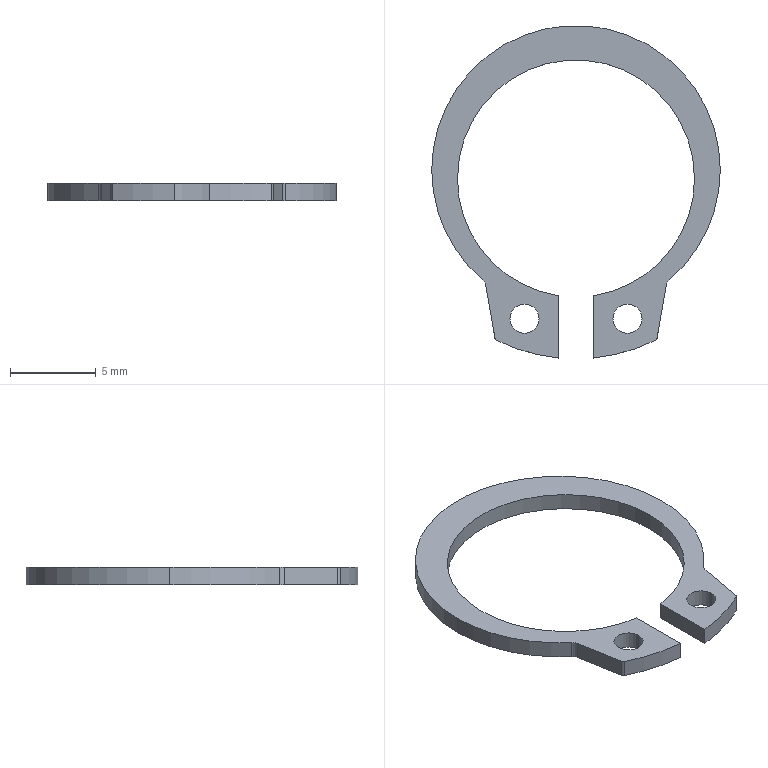Part | SolidWorks | features Fillet 2, Extrusion 1 | 1 solid | 22 faces | box 16.8 x 19.352 x 1 mm | volume 87.473 mm3 | cylinder 16 | plane 6 | commonest cylinder face diameters 1.7 x4 13.8 x3 16.8 x3 0.4 x2 1 x2 21 x2
STEP:
#1=CARTESIAN_POINT('',(2.15,-8.666,-1.));
#2=VERTEX_POINT('',#1);
#3=CARTESIAN_POINT('',(3.85,-8.666,-1.));
#4=VERTEX_POINT('',#3);
#5=CARTESIAN_POINT('',(3.,-8.666,-1.));
#6=DIRECTION('',(0.,0.,1.));
#7=DIRECTION('',(-1.,0.,0.));
#8=AXIS2_PLACEMENT_3D('',#5,#6,#7);
#9=CIRCLE('',#8,0.85);
#10=EDGE_CURVE('',#2,#4,#9,.T.);
#11=ORIENTED_EDGE('',*,*,#10,.F.);
#12=CARTESIAN_POINT('',(2.15,-8.666,0.));
#13=VERTEX_POINT('',#12);
#14=CARTESIAN_POINT('',(2.15,-8.666,-1.));
#15=DIRECTION('',(0.,0.,1.));
#16=VECTOR('',#15,1000.);
#17=LINE('',#14,#16);
#18=EDGE_CURVE('',#2,#13,#17,.T.);
#19=ORIENTED_EDGE('',*,*,#18,.T.);
#20=CARTESIAN_POINT('',(3.85,-8.666,0.));
#21=VERTEX_POINT('',#20);
#22=CARTESIAN_POINT('',(3.,-8.666,0.));
#23=DIRECTION('',(0.,0.,1.));
#24=DIRECTION('',(-1.,0.,0.));
#25=AXIS2_PLACEMENT_3D('',#22,#23,#24);
#26=CIRCLE('',#25,0.85);
#27=EDGE_CURVE('',#13,#21,#26,.T.);
#28=ORIENTED_EDGE('',*,*,#27,.T.);
#29=CARTESIAN_POINT('',(3.85,-8.666,-1.));
#30=DIRECTION('',(0.,0.,1.));
#31=VECTOR('',#30,1000.);
#32=LINE('',#29,#31);
#33=EDGE_CURVE('',#4,#21,#32,.T.);
#34=ORIENTED_EDGE('',*,*,#33,.F.);
#35=EDGE_LOOP('',(#11,#19,#28,#34));
#36=FACE_OUTER_BOUND('',#35,.T.);
#37=CARTESIAN_POINT('',(3.,-8.666,-1.));
#38=DIRECTION('',(0.,0.,1.));
#39=DIRECTION('',(1.,0.,0.));
#40=AXIS2_PLACEMENT_3D('',#37,#38,#39);
#41=CYLINDRICAL_SURFACE('',#40,0.85);
#42=ADVANCED_FACE('',(#36),#41,.F.);
#43=CARTESIAN_POINT('',(-3.85,-8.666,-1.));
#44=VERTEX_POINT('',#43);
#45=CARTESIAN_POINT('',(-2.15,-8.666,-1.));
#46=VERTEX_POINT('',#45);
#47=CARTESIAN_POINT('',(-3.,-8.666,-1.));
#48=DIRECTION('',(0.,0.,1.));
#49=DIRECTION('',(1.,0.,0.));
#50=AXIS2_PLACEMENT_3D('',#47,#48,#49);
#51=CIRCLE('',#50,0.85);
#52=EDGE_CURVE('',#44,#46,#51,.T.);
#53=ORIENTED_EDGE('',*,*,#52,.F.);
#54=CARTESIAN_POINT('',(-3.85,-8.666,0.));
#55=VERTEX_POINT('',#54);
#56=CARTESIAN_POINT('',(-3.85,-8.666,-1.));
#57=DIRECTION('',(0.,0.,1.));
#58=VECTOR('',#57,1000.);
#59=LINE('',#56,#58);
#60=EDGE_CURVE('',#44,#55,#59,.T.);
#61=ORIENTED_EDGE('',*,*,#60,.T.);
#62=CARTESIAN_POINT('',(-2.15,-8.666,0.));
#63=VERTEX_POINT('',#62);
#64=CARTESIAN_POINT('',(-3.,-8.666,0.));
#65=DIRECTION('',(0.,0.,1.));
#66=DIRECTION('',(1.,0.,0.));
#67=AXIS2_PLACEMENT_3D('',#64,#65,#66);
#68=CIRCLE('',#67,0.85);
#69=EDGE_CURVE('',#55,#63,#68,.T.);
#70=ORIENTED_EDGE('',*,*,#69,.T.);
#71=CARTESIAN_POINT('',(-2.15,-8.666,-1.));
#72=DIRECTION('',(0.,0.,1.));
#73=VECTOR('',#72,1000.);
#74=LINE('',#71,#73);
#75=EDGE_CURVE('',#46,#63,#74,.T.);
#76=ORIENTED_EDGE('',*,*,#75,.F.);
#77=EDGE_LOOP('',(#53,#61,#70,#76));
#78=FACE_OUTER_BOUND('',#77,.T.);
#79=CARTESIAN_POINT('',(-3.,-8.666,-1.));
#80=DIRECTION('',(0.,0.,1.));
#81=DIRECTION('',(1.,0.,0.));
#82=AXIS2_PLACEMENT_3D('',#79,#80,#81);
#83=CYLINDRICAL_SURFACE('',#82,0.85);
#84=ADVANCED_FACE('',(#78),#83,.F.);
#85=CARTESIAN_POINT('',(8.4,0.,-1.));
#86=VERTEX_POINT('',#85);
#87=CARTESIAN_POINT('',(-8.4,0.,-1.));
#88=VERTEX_POINT('',#87);
#89=CARTESIAN_POINT('',(0.,0.,-1.));
#90=DIRECTION('',(0.,0.,1.));
#91=DIRECTION('',(1.,0.,0.));
#92=AXIS2_PLACEMENT_3D('',#89,#90,#91);
#93=CIRCLE('',#92,8.4);
#94=EDGE_CURVE('',#86,#88,#93,.T.);
#95=ORIENTED_EDGE('',*,*,#94,.T.);
#96=CARTESIAN_POINT('',(-8.4,0.,0.));
#97=VERTEX_POINT('',#96);
#98=CARTESIAN_POINT('',(-8.4,0.,-1.));
#99=DIRECTION('',(0.,0.,1.));
#100=VECTOR('',#99,1000.);
#101=LINE('',#98,#100);
#102=EDGE_CURVE('',#88,#97,#101,.T.);
#103=ORIENTED_EDGE('',*,*,#102,.T.);
#104=CARTESIAN_POINT('',(8.4,0.,0.));
#105=VERTEX_POINT('',#104);
#106=CARTESIAN_POINT('',(0.,0.,0.));
#107=DIRECTION('',(0.,0.,1.));
#108=DIRECTION('',(1.,0.,0.));
#109=AXIS2_PLACEMENT_3D('',#106,#107,#108);
#110=CIRCLE('',#109,8.4);
#111=EDGE_CURVE('',#105,#97,#110,.T.);
#112=ORIENTED_EDGE('',*,*,#111,.F.);
#113=CARTESIAN_POINT('',(8.4,0.,-1.));
#114=DIRECTION('',(0.,0.,1.));
#115=VECTOR('',#114,1000.);
#116=LINE('',#113,#115);
#117=EDGE_CURVE('',#86,#105,#116,.T.);
#118=ORIENTED_EDGE('',*,*,#117,.F.);
#119=EDGE_LOOP('',(#95,#103,#112,#118));
#120=FACE_OUTER_BOUND('',#119,.T.);
#121=CARTESIAN_POINT('',(0.,0.,-1.));
#122=DIRECTION('',(0.,0.,1.));
#123=DIRECTION('',(1.,0.,0.));
#124=AXIS2_PLACEMENT_3D('',#121,#122,#123);
#125=CYLINDRICAL_SURFACE('',#124,8.4);
#126=ADVANCED_FACE('',(#120),#125,.T.);
#127=CARTESIAN_POINT('',(5.434,-6.406,-1.));
#128=VERTEX_POINT('',#127);
#129=CARTESIAN_POINT('',(0.,0.,-1.));
#130=DIRECTION('',(0.,0.,1.));
#131=DIRECTION('',(1.,0.,0.));
#132=AXIS2_PLACEMENT_3D('',#129,#130,#131);
#133=CIRCLE('',#132,8.4);
#134=EDGE_CURVE('',#128,#86,#133,.T.);
#135=ORIENTED_EDGE('',*,*,#134,.T.);
#136=ORIENTED_EDGE('',*,*,#117,.T.);
#137=CARTESIAN_POINT('',(5.434,-6.406,0.));
#138=VERTEX_POINT('',#137);
#139=CARTESIAN_POINT('',(0.,0.,0.));
#140=DIRECTION('',(0.,0.,1.));
#141=DIRECTION('',(1.,0.,0.));
#142=AXIS2_PLACEMENT_3D('',#139,#140,#141);
#143=CIRCLE('',#142,8.4);
#144=EDGE_CURVE('',#138,#105,#143,.T.);
#145=ORIENTED_EDGE('',*,*,#144,.F.);
#146=CARTESIAN_POINT('',(5.434,-6.406,-1.));
#147=DIRECTION('',(0.,0.,-1.));
#148=VECTOR('',#147,1000.);
#149=LINE('',#146,#148);
#150=EDGE_CURVE('',#138,#128,#149,.T.);
#151=ORIENTED_EDGE('',*,*,#150,.T.);
#152=EDGE_LOOP('',(#135,#136,#145,#151));
#153=FACE_OUTER_BOUND('',#152,.T.);
#154=CARTESIAN_POINT('',(0.,0.,-1.));
#155=DIRECTION('',(0.,0.,1.));
#156=DIRECTION('',(1.,0.,0.));
#157=AXIS2_PLACEMENT_3D('',#154,#155,#156);
#158=CYLINDRICAL_SURFACE('',#157,8.4);
#159=ADVANCED_FACE('',(#153),#158,.T.);
#160=CARTESIAN_POINT('',(-1.,-7.327,-1.));
#161=VERTEX_POINT('',#160);
#162=CARTESIAN_POINT('',(-6.9,-0.5,-1.));
#163=VERTEX_POINT('',#162);
#164=CARTESIAN_POINT('',(0.,-0.5,-1.));
#165=DIRECTION('',(0.,0.,-1.));
#166=DIRECTION('',(1.,0.,0.));
#167=AXIS2_PLACEMENT_3D('',#164,#165,#166);
#168=CIRCLE('',#167,6.9);
#169=EDGE_CURVE('',#161,#163,#168,.T.);
#170=ORIENTED_EDGE('',*,*,#169,.T.);
#171=CARTESIAN_POINT('',(-6.9,-0.5,0.));
#172=VERTEX_POINT('',#171);
#173=CARTESIAN_POINT('',(-6.9,-0.5,-1.));
#174=DIRECTION('',(0.,0.,1.));
#175=VECTOR('',#174,1000.);
#176=LINE('',#173,#175);
#177=EDGE_CURVE('',#163,#172,#176,.T.);
#178=ORIENTED_EDGE('',*,*,#177,.T.);
#179=CARTESIAN_POINT('',(-1.,-7.327,0.));
#180=VERTEX_POINT('',#179);
#181=CARTESIAN_POINT('',(0.,-0.5,0.));
#182=DIRECTION('',(0.,0.,-1.));
#183=DIRECTION('',(1.,0.,0.));
#184=AXIS2_PLACEMENT_3D('',#181,#182,#183);
#185=CIRCLE('',#184,6.9);
#186=EDGE_CURVE('',#180,#172,#185,.T.);
#187=ORIENTED_EDGE('',*,*,#186,.F.);
#188=CARTESIAN_POINT('',(-1.,-7.327,-1.));
#189=DIRECTION('',(0.,0.,1.));
#190=VECTOR('',#189,1000.);
#191=LINE('',#188,#190);
#192=EDGE_CURVE('',#161,#180,#191,.T.);
#193=ORIENTED_EDGE('',*,*,#192,.F.);
#194=EDGE_LOOP('',(#170,#178,#187,#193));
#195=FACE_OUTER_BOUND('',#194,.T.);
#196=CARTESIAN_POINT('',(0.,-0.5,-1.));
#197=DIRECTION('',(0.,0.,1.));
#198=DIRECTION('',(1.,0.,0.));
#199=AXIS2_PLACEMENT_3D('',#196,#197,#198);
#200=CYLINDRICAL_SURFACE('',#199,6.9);
#201=ADVANCED_FACE('',(#195),#200,.F.);
#202=ORIENTED_EDGE('',*,*,#177,.F.);
#203=CARTESIAN_POINT('',(6.9,-0.5,-1.));
#204=VERTEX_POINT('',#203);
#205=CARTESIAN_POINT('',(0.,-0.5,-1.));
#206=DIRECTION('',(0.,0.,-1.));
#207=DIRECTION('',(1.,0.,0.));
#208=AXIS2_PLACEMENT_3D('',#205,#206,#207);
#209=CIRCLE('',#208,6.9);
#210=EDGE_CURVE('',#163,#204,#209,.T.);
#211=ORIENTED_EDGE('',*,*,#210,.T.);
#212=CARTESIAN_POINT('',(6.9,-0.5,0.));
#213=VERTEX_POINT('',#212);
#214=CARTESIAN_POINT('',(6.9,-0.5,-1.));
#215=DIRECTION('',(0.,0.,1.));
#216=VECTOR('',#215,1000.);
#217=LINE('',#214,#216);
#218=EDGE_CURVE('',#204,#213,#217,.T.);
#219=ORIENTED_EDGE('',*,*,#218,.T.);
#220=CARTESIAN_POINT('',(0.,-0.5,0.));
#221=DIRECTION('',(0.,0.,-1.));
#222=DIRECTION('',(1.,0.,0.));
#223=AXIS2_PLACEMENT_3D('',#220,#221,#222);
#224=CIRCLE('',#223,6.9);
#225=EDGE_CURVE('',#172,#213,#224,.T.);
#226=ORIENTED_EDGE('',*,*,#225,.F.);
#227=EDGE_LOOP('',(#202,#211,#219,#226));
#228=FACE_OUTER_BOUND('',#227,.T.);
#229=CARTESIAN_POINT('',(0.,-0.5,-1.));
#230=DIRECTION('',(0.,0.,1.));
#231=DIRECTION('',(1.,0.,0.));
#232=AXIS2_PLACEMENT_3D('',#229,#230,#231);
#233=CYLINDRICAL_SURFACE('',#232,6.9);
#234=ADVANCED_FACE('',(#228),#233,.F.);
#235=CARTESIAN_POINT('',(1.,-10.952,-1.));
#236=VERTEX_POINT('',#235);
#237=CARTESIAN_POINT('',(4.611,-9.933,-1.));
#238=VERTEX_POINT('',#237);
#239=CARTESIAN_POINT('',(0.,-0.5,-1.));
#240=DIRECTION('',(0.,0.,1.));
#241=DIRECTION('',(-1.,0.,0.));
#242=AXIS2_PLACEMENT_3D('',#239,#240,#241);
#243=CIRCLE('',#242,10.5);
#244=EDGE_CURVE('',#236,#238,#243,.T.);
#245=ORIENTED_EDGE('',*,*,#244,.T.);
#246=CARTESIAN_POINT('',(4.611,-9.933,0.));
#247=VERTEX_POINT('',#246);
#248=CARTESIAN_POINT('',(4.611,-9.933,-1.));
#249=DIRECTION('',(0.,0.,1.));
#250=VECTOR('',#249,1000.);
#251=LINE('',#248,#250);
#252=EDGE_CURVE('',#238,#247,#251,.T.);
#253=ORIENTED_EDGE('',*,*,#252,.T.);
#254=CARTESIAN_POINT('',(1.,-10.952,0.));
#255=VERTEX_POINT('',#254);
#256=CARTESIAN_POINT('',(0.,-0.5,0.));
#257=DIRECTION('',(0.,0.,1.));
#258=DIRECTION('',(-1.,0.,0.));
#259=AXIS2_PLACEMENT_3D('',#256,#257,#258);
#260=CIRCLE('',#259,10.5);
#261=EDGE_CURVE('',#255,#247,#260,.T.);
#262=ORIENTED_EDGE('',*,*,#261,.F.);
#263=CARTESIAN_POINT('',(1.,-10.952,-1.));
#264=DIRECTION('',(0.,0.,1.));
#265=VECTOR('',#264,1000.);
#266=LINE('',#263,#265);
#267=EDGE_CURVE('',#236,#255,#266,.T.);
#268=ORIENTED_EDGE('',*,*,#267,.F.);
#269=EDGE_LOOP('',(#245,#253,#262,#268));
#270=FACE_OUTER_BOUND('',#269,.T.);
#271=CARTESIAN_POINT('',(0.,-0.5,-1.));
#272=DIRECTION('',(0.,0.,1.));
#273=DIRECTION('',(1.,0.,0.));
#274=AXIS2_PLACEMENT_3D('',#271,#272,#273);
#275=CYLINDRICAL_SURFACE('',#274,10.5);
#276=ADVANCED_FACE('',(#270),#275,.T.);
#277=CARTESIAN_POINT('',(1.,-7.327,0.));
#278=VERTEX_POINT('',#277);
#279=CARTESIAN_POINT('',(1.,-7.327,0.));
#280=DIRECTION('',(0.,-1.,0.));
#281=VECTOR('',#280,1000.);
#282=LINE('',#279,#281);
#283=EDGE_CURVE('',#278,#255,#282,.T.);
#284=ORIENTED_EDGE('',*,*,#283,.F.);
#285=CARTESIAN_POINT('',(1.,-7.327,-1.));
#286=VERTEX_POINT('',#285);
#287=CARTESIAN_POINT('',(1.,-7.327,-1.));
#288=DIRECTION('',(0.,0.,1.));
#289=VECTOR('',#288,1000.);
#290=LINE('',#287,#289);
#291=EDGE_CURVE('',#286,#278,#290,.T.);
#292=ORIENTED_EDGE('',*,*,#291,.F.);
#293=CARTESIAN_POINT('',(1.,-7.327,-1.));
#294=DIRECTION('',(0.,-1.,0.));
#295=VECTOR('',#294,1000.);
#296=LINE('',#293,#295);
#297=EDGE_CURVE('',#286,#236,#296,.T.);
#298=ORIENTED_EDGE('',*,*,#297,.T.);
#299=ORIENTED_EDGE('',*,*,#267,.T.);
#300=EDGE_LOOP('',(#284,#292,#298,#299));
#301=FACE_OUTER_BOUND('',#300,.T.);
#302=CARTESIAN_POINT('',(1.,-7.327,-1.));
#303=DIRECTION('',(-1.,0.,0.));
#304=DIRECTION('',(0.,-1.,0.));
#305=AXIS2_PLACEMENT_3D('',#302,#303,#304);
#306=PLANE('',#305);
#307=ADVANCED_FACE('',(#301),#306,.T.);
#308=ORIENTED_EDGE('',*,*,#218,.F.);
#309=CARTESIAN_POINT('',(0.,-0.5,-1.));
#310=DIRECTION('',(0.,0.,-1.));
#311=DIRECTION('',(1.,0.,0.));
#312=AXIS2_PLACEMENT_3D('',#309,#310,#311);
#313=CIRCLE('',#312,6.9);
#314=EDGE_CURVE('',#204,#286,#313,.T.);
#315=ORIENTED_EDGE('',*,*,#314,.T.);
#316=ORIENTED_EDGE('',*,*,#291,.T.);
#317=CARTESIAN_POINT('',(0.,-0.5,0.));
#318=DIRECTION('',(0.,0.,-1.));
#319=DIRECTION('',(1.,0.,0.));
#320=AXIS2_PLACEMENT_3D('',#317,#318,#319);
#321=CIRCLE('',#320,6.9);
#322=EDGE_CURVE('',#213,#278,#321,.T.);
#323=ORIENTED_EDGE('',*,*,#322,.F.);
#324=EDGE_LOOP('',(#308,#315,#316,#323));
#325=FACE_OUTER_BOUND('',#324,.T.);
#326=CARTESIAN_POINT('',(0.,-0.5,-1.));
#327=DIRECTION('',(0.,0.,1.));
#328=DIRECTION('',(1.,0.,0.));
#329=AXIS2_PLACEMENT_3D('',#326,#327,#328);
#330=CYLINDRICAL_SURFACE('',#329,6.9);
#331=ADVANCED_FACE('',(#325),#330,.F.);
#332=CARTESIAN_POINT('',(-1.,-10.952,0.));
#333=VERTEX_POINT('',#332);
#334=CARTESIAN_POINT('',(-1.,-7.327,0.));
#335=DIRECTION('',(0.,1.,0.));
#336=VECTOR('',#335,1000.);
#337=LINE('',#334,#336);
#338=EDGE_CURVE('',#333,#180,#337,.T.);
#339=ORIENTED_EDGE('',*,*,#338,.F.);
#340=CARTESIAN_POINT('',(-1.,-10.952,-1.));
#341=VERTEX_POINT('',#340);
#342=CARTESIAN_POINT('',(-1.,-10.952,-1.));
#343=DIRECTION('',(0.,0.,1.));
#344=VECTOR('',#343,1000.);
#345=LINE('',#342,#344);
#346=EDGE_CURVE('',#341,#333,#345,.T.);
#347=ORIENTED_EDGE('',*,*,#346,.F.);
#348=CARTESIAN_POINT('',(-1.,-7.327,-1.));
#349=DIRECTION('',(0.,1.,0.));
#350=VECTOR('',#349,1000.);
#351=LINE('',#348,#350);
#352=EDGE_CURVE('',#341,#161,#351,.T.);
#353=ORIENTED_EDGE('',*,*,#352,.T.);
#354=ORIENTED_EDGE('',*,*,#192,.T.);
#355=EDGE_LOOP('',(#339,#347,#353,#354));
#356=FACE_OUTER_BOUND('',#355,.T.);
#357=CARTESIAN_POINT('',(-1.,-7.327,-1.));
#358=DIRECTION('',(1.,0.,0.));
#359=DIRECTION('',(0.,1.,0.));
#360=AXIS2_PLACEMENT_3D('',#357,#358,#359);
#361=PLANE('',#360);
#362=ADVANCED_FACE('',(#356),#361,.T.);
#363=CARTESIAN_POINT('',(-4.611,-9.933,0.));
#364=VERTEX_POINT('',#363);
#365=CARTESIAN_POINT('',(0.,-0.5,0.));
#366=DIRECTION('',(0.,0.,1.));
#367=DIRECTION('',(1.,0.,0.));
#368=AXIS2_PLACEMENT_3D('',#365,#366,#367);
#369=CIRCLE('',#368,10.5);
#370=EDGE_CURVE('',#364,#333,#369,.T.);
#371=ORIENTED_EDGE('',*,*,#370,.F.);
#372=CARTESIAN_POINT('',(-4.611,-9.933,-1.));
#373=VERTEX_POINT('',#372);
#374=CARTESIAN_POINT('',(-4.611,-9.933,-1.));
#375=DIRECTION('',(0.,0.,-1.));
#376=VECTOR('',#375,1000.);
#377=LINE('',#374,#376);
#378=EDGE_CURVE('',#364,#373,#377,.T.);
#379=ORIENTED_EDGE('',*,*,#378,.T.);
#380=CARTESIAN_POINT('',(0.,-0.5,-1.));
#381=DIRECTION('',(0.,0.,1.));
#382=DIRECTION('',(1.,0.,0.));
#383=AXIS2_PLACEMENT_3D('',#380,#381,#382);
#384=CIRCLE('',#383,10.5);
#385=EDGE_CURVE('',#373,#341,#384,.T.);
#386=ORIENTED_EDGE('',*,*,#385,.T.);
#387=ORIENTED_EDGE('',*,*,#346,.T.);
#388=EDGE_LOOP('',(#371,#379,#386,#387));
#389=FACE_OUTER_BOUND('',#388,.T.);
#390=CARTESIAN_POINT('',(0.,-0.5,-1.));
#391=DIRECTION('',(0.,0.,1.));
#392=DIRECTION('',(1.,0.,0.));
#393=AXIS2_PLACEMENT_3D('',#390,#391,#392);
#394=CYLINDRICAL_SURFACE('',#393,10.5);
#395=ADVANCED_FACE('',(#389),#394,.T.);
#396=CARTESIAN_POINT('',(-5.265,-6.7,0.));
#397=VERTEX_POINT('',#396);
#398=CARTESIAN_POINT('',(-4.721,-9.788,0.));
#399=VERTEX_POINT('',#398);
#400=CARTESIAN_POINT('',(-5.297,-6.519,0.));
#401=DIRECTION('',(0.1736,-0.9848,0.));
#402=VECTOR('',#401,1000.);
#403=LINE('',#400,#402);
#404=EDGE_CURVE('',#397,#399,#403,.T.);
#405=ORIENTED_EDGE('',*,*,#404,.F.);
#406=CARTESIAN_POINT('',(-5.265,-6.7,-1.));
#407=VERTEX_POINT('',#406);
#408=CARTESIAN_POINT('',(-5.265,-6.7,-1.));
#409=DIRECTION('',(0.,0.,-1.));
#410=VECTOR('',#409,1000.);
#411=LINE('',#408,#410);
#412=EDGE_CURVE('',#397,#407,#411,.T.);
#413=ORIENTED_EDGE('',*,*,#412,.T.);
#414=CARTESIAN_POINT('',(-4.721,-9.788,-1.));
#415=VERTEX_POINT('',#414);
#416=CARTESIAN_POINT('',(-5.297,-6.519,-1.));
#417=DIRECTION('',(0.1736,-0.9848,0.));
#418=VECTOR('',#417,1000.);
#419=LINE('',#416,#418);
#420=EDGE_CURVE('',#407,#415,#419,.T.);
#421=ORIENTED_EDGE('',*,*,#420,.T.);
#422=CARTESIAN_POINT('',(-4.721,-9.788,-1.));
#423=DIRECTION('',(0.,0.,1.));
#424=VECTOR('',#423,1000.);
#425=LINE('',#422,#424);
#426=EDGE_CURVE('',#415,#399,#425,.T.);
#427=ORIENTED_EDGE('',*,*,#426,.T.);
#428=EDGE_LOOP('',(#405,#413,#421,#427));
#429=FACE_OUTER_BOUND('',#428,.T.);
#430=CARTESIAN_POINT('',(-5.297,-6.519,-1.));
#431=DIRECTION('',(-0.9848,-0.1736,0.));
#432=DIRECTION('',(0.1736,-0.9848,0.));
#433=AXIS2_PLACEMENT_3D('',#430,#431,#432);
#434=PLANE('',#433);
#435=ADVANCED_FACE('',(#429),#434,.T.);
#436=ORIENTED_EDGE('',*,*,#102,.F.);
#437=CARTESIAN_POINT('',(-5.434,-6.406,-1.));
#438=VERTEX_POINT('',#437);
#439=CARTESIAN_POINT('',(0.,0.,-1.));
#440=DIRECTION('',(0.,0.,1.));
#441=DIRECTION('',(1.,0.,0.));
#442=AXIS2_PLACEMENT_3D('',#439,#440,#441);
#443=CIRCLE('',#442,8.4);
#444=EDGE_CURVE('',#88,#438,#443,.T.);
#445=ORIENTED_EDGE('',*,*,#444,.T.);
#446=CARTESIAN_POINT('',(-5.434,-6.406,0.));
#447=VERTEX_POINT('',#446);
#448=CARTESIAN_POINT('',(-5.434,-6.406,-1.));
#449=DIRECTION('',(0.,0.,1.));
#450=VECTOR('',#449,1000.);
#451=LINE('',#448,#450);
#452=EDGE_CURVE('',#438,#447,#451,.T.);
#453=ORIENTED_EDGE('',*,*,#452,.T.);
#454=CARTESIAN_POINT('',(0.,0.,0.));
#455=DIRECTION('',(0.,0.,1.));
#456=DIRECTION('',(1.,0.,0.));
#457=AXIS2_PLACEMENT_3D('',#454,#455,#456);
#458=CIRCLE('',#457,8.4);
#459=EDGE_CURVE('',#97,#447,#458,.T.);
#460=ORIENTED_EDGE('',*,*,#459,.F.);
#461=EDGE_LOOP('',(#436,#445,#453,#460));
#462=FACE_OUTER_BOUND('',#461,.T.);
#463=CARTESIAN_POINT('',(0.,0.,-1.));
#464=DIRECTION('',(0.,0.,1.));
#465=DIRECTION('',(1.,0.,0.));
#466=AXIS2_PLACEMENT_3D('',#463,#464,#465);
#467=CYLINDRICAL_SURFACE('',#466,8.4);
#468=ADVANCED_FACE('',(#462),#467,.T.);
#469=CARTESIAN_POINT('',(4.721,-9.788,-1.));
#470=VERTEX_POINT('',#469);
#471=CARTESIAN_POINT('',(5.265,-6.7,-1.));
#472=VERTEX_POINT('',#471);
#473=CARTESIAN_POINT('',(5.297,-6.519,-1.));
#474=DIRECTION('',(0.1736,0.9848,0.));
#475=VECTOR('',#474,1000.);
#476=LINE('',#473,#475);
#477=EDGE_CURVE('',#470,#472,#476,.T.);
#478=ORIENTED_EDGE('',*,*,#477,.T.);
#479=CARTESIAN_POINT('',(5.265,-6.7,0.));
#480=VERTEX_POINT('',#479);
#481=CARTESIAN_POINT('',(5.265,-6.7,0.));
#482=DIRECTION('',(0.,0.,1.));
#483=VECTOR('',#482,1000.);
#484=LINE('',#481,#483);
#485=EDGE_CURVE('',#472,#480,#484,.T.);
#486=ORIENTED_EDGE('',*,*,#485,.T.);
#487=CARTESIAN_POINT('',(4.721,-9.788,0.));
#488=VERTEX_POINT('',#487);
#489=CARTESIAN_POINT('',(5.297,-6.519,0.));
#490=DIRECTION('',(0.1736,0.9848,0.));
#491=VECTOR('',#490,1000.);
#492=LINE('',#489,#491);
#493=EDGE_CURVE('',#488,#480,#492,.T.);
#494=ORIENTED_EDGE('',*,*,#493,.F.);
#495=CARTESIAN_POINT('',(4.721,-9.788,-1.));
#496=DIRECTION('',(0.,0.,-1.));
#497=VECTOR('',#496,1000.);
#498=LINE('',#495,#497);
#499=EDGE_CURVE('',#488,#470,#498,.T.);
#500=ORIENTED_EDGE('',*,*,#499,.T.);
#501=EDGE_LOOP('',(#478,#486,#494,#500));
#502=FACE_OUTER_BOUND('',#501,.T.);
#503=CARTESIAN_POINT('',(5.297,-6.519,-1.));
#504=DIRECTION('',(0.9848,-0.1736,0.));
#505=DIRECTION('',(0.1736,0.9848,0.));
#506=AXIS2_PLACEMENT_3D('',#503,#504,#505);
#507=PLANE('',#506);
#508=ADVANCED_FACE('',(#502),#507,.T.);
#509=CARTESIAN_POINT('',(3.,-8.666,-1.));
#510=DIRECTION('',(0.,0.,1.));
#511=DIRECTION('',(-1.,0.,0.));
#512=AXIS2_PLACEMENT_3D('',#509,#510,#511);
#513=CIRCLE('',#512,0.85);
#514=EDGE_CURVE('',#4,#2,#513,.T.);
#515=ORIENTED_EDGE('',*,*,#514,.T.);
#516=ORIENTED_EDGE('',*,*,#10,.T.);
#517=EDGE_LOOP('',(#515,#516));
#518=FACE_BOUND('',#517,.T.);
#519=CARTESIAN_POINT('',(-3.,-8.666,-1.));
#520=DIRECTION('',(0.,0.,1.));
#521=DIRECTION('',(1.,0.,0.));
#522=AXIS2_PLACEMENT_3D('',#519,#520,#521);
#523=CIRCLE('',#522,0.85);
#524=EDGE_CURVE('',#46,#44,#523,.T.);
#525=ORIENTED_EDGE('',*,*,#524,.T.);
#526=ORIENTED_EDGE('',*,*,#52,.T.);
#527=EDGE_LOOP('',(#525,#526));
#528=FACE_BOUND('',#527,.T.);
#529=ORIENTED_EDGE('',*,*,#385,.F.);
#530=CARTESIAN_POINT('',(-4.524,-9.753,-1.));
#531=DIRECTION('',(0.,0.,-1.));
#532=DIRECTION('',(-1.,0.,0.));
#533=AXIS2_PLACEMENT_3D('',#530,#531,#532);
#534=CIRCLE('',#533,0.2);
#535=EDGE_CURVE('',#373,#415,#534,.T.);
#536=ORIENTED_EDGE('',*,*,#535,.T.);
#537=ORIENTED_EDGE('',*,*,#420,.F.);
#538=CARTESIAN_POINT('',(-5.758,-6.787,-1.));
#539=DIRECTION('',(0.,0.,1.));
#540=DIRECTION('',(-1.,0.,0.));
#541=AXIS2_PLACEMENT_3D('',#538,#539,#540);
#542=CIRCLE('',#541,0.5);
#543=EDGE_CURVE('',#407,#438,#542,.T.);
#544=ORIENTED_EDGE('',*,*,#543,.T.);
#545=ORIENTED_EDGE('',*,*,#444,.F.);
#546=ORIENTED_EDGE('',*,*,#94,.F.);
#547=ORIENTED_EDGE('',*,*,#134,.F.);
#548=CARTESIAN_POINT('',(5.758,-6.787,-1.));
#549=DIRECTION('',(0.,0.,1.));
#550=DIRECTION('',(-1.,0.,0.));
#551=AXIS2_PLACEMENT_3D('',#548,#549,#550);
#552=CIRCLE('',#551,0.5);
#553=EDGE_CURVE('',#128,#472,#552,.T.);
#554=ORIENTED_EDGE('',*,*,#553,.T.);
#555=ORIENTED_EDGE('',*,*,#477,.F.);
#556=CARTESIAN_POINT('',(4.524,-9.753,-1.));
#557=DIRECTION('',(0.,0.,-1.));
#558=DIRECTION('',(-1.,0.,0.));
#559=AXIS2_PLACEMENT_3D('',#556,#557,#558);
#560=CIRCLE('',#559,0.2);
#561=EDGE_CURVE('',#470,#238,#560,.T.);
#562=ORIENTED_EDGE('',*,*,#561,.T.);
#563=ORIENTED_EDGE('',*,*,#244,.F.);
#564=ORIENTED_EDGE('',*,*,#297,.F.);
#565=ORIENTED_EDGE('',*,*,#314,.F.);
#566=ORIENTED_EDGE('',*,*,#210,.F.);
#567=ORIENTED_EDGE('',*,*,#169,.F.);
#568=ORIENTED_EDGE('',*,*,#352,.F.);
#569=EDGE_LOOP('',(#529,#536,#537,#544,#545,#546,#547,#554,#555,#562,#563,#564,#565,#566,#567,#568));
#570=FACE_OUTER_BOUND('',#569,.T.);
#571=CARTESIAN_POINT('',(0.,-0.5,-1.));
#572=DIRECTION('',(0.,0.,-1.));
#573=DIRECTION('',(-1.,0.,0.));
#574=AXIS2_PLACEMENT_3D('',#571,#572,#573);
#575=PLANE('',#574);
#576=ADVANCED_FACE('',(#518,#528,#570),#575,.T.);
#577=CARTESIAN_POINT('',(3.,-8.666,0.));
#578=DIRECTION('',(0.,0.,1.));
#579=DIRECTION('',(-1.,0.,0.));
#580=AXIS2_PLACEMENT_3D('',#577,#578,#579);
#581=CIRCLE('',#580,0.85);
#582=EDGE_CURVE('',#21,#13,#581,.T.);
#583=ORIENTED_EDGE('',*,*,#582,.F.);
#584=ORIENTED_EDGE('',*,*,#27,.F.);
#585=EDGE_LOOP('',(#583,#584));
#586=FACE_BOUND('',#585,.T.);
#587=CARTESIAN_POINT('',(-3.,-8.666,0.));
#588=DIRECTION('',(0.,0.,1.));
#589=DIRECTION('',(1.,0.,0.));
#590=AXIS2_PLACEMENT_3D('',#587,#588,#589);
#591=CIRCLE('',#590,0.85);
#592=EDGE_CURVE('',#63,#55,#591,.T.);
#593=ORIENTED_EDGE('',*,*,#592,.F.);
#594=ORIENTED_EDGE('',*,*,#69,.F.);
#595=EDGE_LOOP('',(#593,#594));
#596=FACE_BOUND('',#595,.T.);
#597=ORIENTED_EDGE('',*,*,#144,.T.);
#598=ORIENTED_EDGE('',*,*,#111,.T.);
#599=ORIENTED_EDGE('',*,*,#459,.T.);
#600=CARTESIAN_POINT('',(-5.758,-6.787,0.));
#601=DIRECTION('',(0.,0.,-1.));
#602=DIRECTION('',(-1.,0.,0.));
#603=AXIS2_PLACEMENT_3D('',#600,#601,#602);
#604=CIRCLE('',#603,0.5);
#605=EDGE_CURVE('',#447,#397,#604,.T.);
#606=ORIENTED_EDGE('',*,*,#605,.T.);
#607=ORIENTED_EDGE('',*,*,#404,.T.);
#608=CARTESIAN_POINT('',(-4.524,-9.753,0.));
#609=DIRECTION('',(0.,0.,1.));
#610=DIRECTION('',(-1.,0.,0.));
#611=AXIS2_PLACEMENT_3D('',#608,#609,#610);
#612=CIRCLE('',#611,0.2);
#613=EDGE_CURVE('',#399,#364,#612,.T.);
#614=ORIENTED_EDGE('',*,*,#613,.T.);
#615=ORIENTED_EDGE('',*,*,#370,.T.);
#616=ORIENTED_EDGE('',*,*,#338,.T.);
#617=ORIENTED_EDGE('',*,*,#186,.T.);
#618=ORIENTED_EDGE('',*,*,#225,.T.);
#619=ORIENTED_EDGE('',*,*,#322,.T.);
#620=ORIENTED_EDGE('',*,*,#283,.T.);
#621=ORIENTED_EDGE('',*,*,#261,.T.);
#622=CARTESIAN_POINT('',(4.524,-9.753,0.));
#623=DIRECTION('',(0.,0.,1.));
#624=DIRECTION('',(-1.,0.,0.));
#625=AXIS2_PLACEMENT_3D('',#622,#623,#624);
#626=CIRCLE('',#625,0.2);
#627=EDGE_CURVE('',#247,#488,#626,.T.);
#628=ORIENTED_EDGE('',*,*,#627,.T.);
#629=ORIENTED_EDGE('',*,*,#493,.T.);
#630=CARTESIAN_POINT('',(5.758,-6.787,0.));
#631=DIRECTION('',(0.,0.,-1.));
#632=DIRECTION('',(-1.,0.,0.));
#633=AXIS2_PLACEMENT_3D('',#630,#631,#632);
#634=CIRCLE('',#633,0.5);
#635=EDGE_CURVE('',#480,#138,#634,.T.);
#636=ORIENTED_EDGE('',*,*,#635,.T.);
#637=EDGE_LOOP('',(#597,#598,#599,#606,#607,#614,#615,#616,#617,#618,#619,#620,#621,#628,#629,#636));
#638=FACE_OUTER_BOUND('',#637,.T.);
#639=CARTESIAN_POINT('',(0.,-0.5,0.));
#640=DIRECTION('',(0.,0.,-1.));
#641=DIRECTION('',(-1.,0.,0.));
#642=AXIS2_PLACEMENT_3D('',#639,#640,#641);
#643=PLANE('',#642);
#644=ADVANCED_FACE('',(#586,#596,#638),#643,.F.);
#645=ORIENTED_EDGE('',*,*,#60,.F.);
#646=ORIENTED_EDGE('',*,*,#524,.F.);
#647=ORIENTED_EDGE('',*,*,#75,.T.);
#648=ORIENTED_EDGE('',*,*,#592,.T.);
#649=EDGE_LOOP('',(#645,#646,#647,#648));
#650=FACE_OUTER_BOUND('',#649,.T.);
#651=CARTESIAN_POINT('',(-3.,-8.666,-1.));
#652=DIRECTION('',(0.,0.,1.));
#653=DIRECTION('',(1.,0.,0.));
#654=AXIS2_PLACEMENT_3D('',#651,#652,#653);
#655=CYLINDRICAL_SURFACE('',#654,0.85);
#656=ADVANCED_FACE('',(#650),#655,.F.);
#657=ORIENTED_EDGE('',*,*,#18,.F.);
#658=ORIENTED_EDGE('',*,*,#514,.F.);
#659=ORIENTED_EDGE('',*,*,#33,.T.);
#660=ORIENTED_EDGE('',*,*,#582,.T.);
#661=EDGE_LOOP('',(#657,#658,#659,#660));
#662=FACE_OUTER_BOUND('',#661,.T.);
#663=CARTESIAN_POINT('',(3.,-8.666,-1.));
#664=DIRECTION('',(0.,0.,1.));
#665=DIRECTION('',(1.,0.,0.));
#666=AXIS2_PLACEMENT_3D('',#663,#664,#665);
#667=CYLINDRICAL_SURFACE('',#666,0.85);
#668=ADVANCED_FACE('',(#662),#667,.F.);
#669=ORIENTED_EDGE('',*,*,#535,.F.);
#670=ORIENTED_EDGE('',*,*,#378,.F.);
#671=ORIENTED_EDGE('',*,*,#613,.F.);
#672=ORIENTED_EDGE('',*,*,#426,.F.);
#673=EDGE_LOOP('',(#669,#670,#671,#672));
#674=FACE_OUTER_BOUND('',#673,.T.);
#675=CARTESIAN_POINT('',(-4.524,-9.753,-1.));
#676=DIRECTION('',(0.,0.,1.));
#677=DIRECTION('',(1.,0.,0.));
#678=AXIS2_PLACEMENT_3D('',#675,#676,#677);
#679=CYLINDRICAL_SURFACE('',#678,0.2);
#680=ADVANCED_FACE('',(#674),#679,.T.);
#681=ORIENTED_EDGE('',*,*,#561,.F.);
#682=ORIENTED_EDGE('',*,*,#499,.F.);
#683=ORIENTED_EDGE('',*,*,#627,.F.);
#684=ORIENTED_EDGE('',*,*,#252,.F.);
#685=EDGE_LOOP('',(#681,#682,#683,#684));
#686=FACE_OUTER_BOUND('',#685,.T.);
#687=CARTESIAN_POINT('',(4.524,-9.753,-1.));
#688=DIRECTION('',(0.,0.,1.));
#689=DIRECTION('',(1.,0.,0.));
#690=AXIS2_PLACEMENT_3D('',#687,#688,#689);
#691=CYLINDRICAL_SURFACE('',#690,0.2);
#692=ADVANCED_FACE('',(#686),#691,.T.);
#693=ORIENTED_EDGE('',*,*,#553,.F.);
#694=ORIENTED_EDGE('',*,*,#150,.F.);
#695=ORIENTED_EDGE('',*,*,#635,.F.);
#696=ORIENTED_EDGE('',*,*,#485,.F.);
#697=EDGE_LOOP('',(#693,#694,#695,#696));
#698=FACE_OUTER_BOUND('',#697,.T.);
#699=CARTESIAN_POINT('',(5.758,-6.787,-1.));
#700=DIRECTION('',(0.,0.,1.));
#701=DIRECTION('',(1.,0.,0.));
#702=AXIS2_PLACEMENT_3D('',#699,#700,#701);
#703=CYLINDRICAL_SURFACE('',#702,0.5);
#704=ADVANCED_FACE('',(#698),#703,.F.);
#705=ORIENTED_EDGE('',*,*,#543,.F.);
#706=ORIENTED_EDGE('',*,*,#412,.F.);
#707=ORIENTED_EDGE('',*,*,#605,.F.);
#708=ORIENTED_EDGE('',*,*,#452,.F.);
#709=EDGE_LOOP('',(#705,#706,#707,#708));
#710=FACE_OUTER_BOUND('',#709,.T.);
#711=CARTESIAN_POINT('',(-5.758,-6.787,-1.));
#712=DIRECTION('',(0.,0.,1.));
#713=DIRECTION('',(1.,0.,0.));
#714=AXIS2_PLACEMENT_3D('',#711,#712,#713);
#715=CYLINDRICAL_SURFACE('',#714,0.5);
#716=ADVANCED_FACE('',(#710),#715,.F.);
#717=CLOSED_SHELL('',(#42,#84,#126,#159,#201,#234,#276,#307,#331,#362,#395,#435,#468,#508,#576,#644,#656,#668,#680,#692,#704,#716));
#718=MANIFOLD_SOLID_BREP('',#717);
#719=CARTESIAN_POINT('',(0.,0.,0.));
#720=DIRECTION('',(0.,0.,1.));
#721=DIRECTION('',(1.,0.,0.));
#722=AXIS2_PLACEMENT_3D('',#719,#720,#721);
#723=(LENGTH_UNIT()NAMED_UNIT(*)SI_UNIT(.MILLI.,.METRE.));
#724=UNCERTAINTY_MEASURE_WITH_UNIT(LENGTH_MEASURE(0.00001),#723,'','');
#725=(NAMED_UNIT(*)PLANE_ANGLE_UNIT()SI_UNIT($,.RADIAN.));
#726=(NAMED_UNIT(*)SI_UNIT($,.STERADIAN.)SOLID_ANGLE_UNIT());
#727=(GEOMETRIC_REPRESENTATION_CONTEXT(3)GLOBAL_UNCERTAINTY_ASSIGNED_CONTEXT((#724))GLOBAL_UNIT_ASSIGNED_CONTEXT((#723,#725,#726))REPRESENTATION_CONTEXT('',''));
#728=ADVANCED_BREP_SHAPE_REPRESENTATION('',(#718,#722),#727);